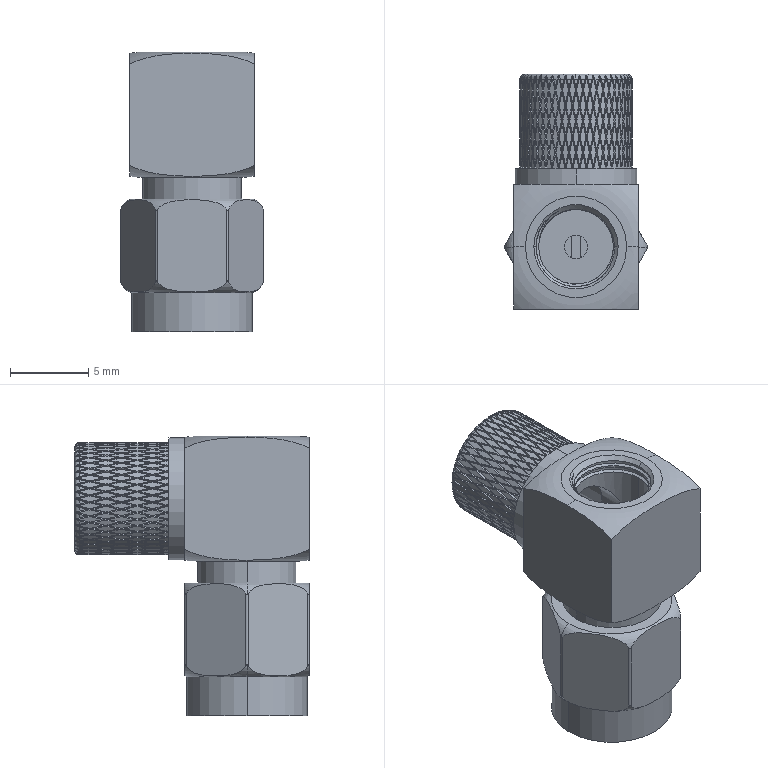Part | SolidWorks | features ICE 11, Helix 3, SweepCut 3, RevCut 2, Chamfer 1, CirPattern 1, Extrusion 1, Fillet 1, MirrorPattern 1, Revolution 1 | 1 solid | 1991 faces | box 9.176 x 15.05 x 17.9 mm | volume 892.261 mm3 | spline 1406 | cylinder 444 | plane 127 | torus 10 | cone 4 | commonest cylinder face diameters 7.2 x404 5.65 x13 0.4 x7 4.8 x4 0.9 x2 1.5 x2